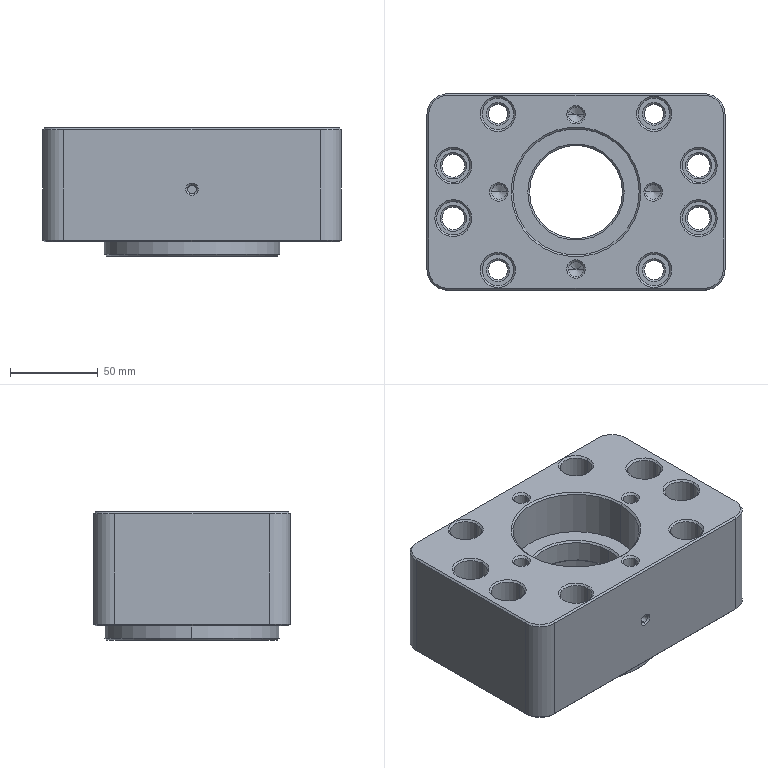NC program | NX | posted with a generic post | part box 170 x 112 x 73 mm
Lines 1 to 69 of 12198:
N10 G17 G21 G94 G90
(DRILLING , TOOL : ZXZ)
N12 T01 M6
N14 G54
N16 G17 G0 G90 X44.5 Y-44.5 S5000 M3
N18 G43 Z30. H1
N20 G94 G81 G98 Z-1. F250. R3.
N22 X70. Y-15.
N24 X44. Y0.
N26 X70. Y15.
N28 X44.5 Y44.5
N30 X0. Y44.
N32 Y0.
N34 Y-44.
N36 X-44.5 Y-44.5
N38 X-70. Y-15.
N40 X-44. Y0.
N42 X-70. Y15.
N44 X-44.5 Y44.5
N46 G80
N48 G0 X-44.5 Y44.5 Z30.
N50 M5
(DRILLING_COPY_COPY_1 , TOOL : 8.5ZT)
N52 T18 M6
N54 G54
N56 G17 G0 G90 X44. Y0. S1573 M3
N58 G43 Z30. H18
N60 G94 G83 G98 Z-28.054 F250. Q2. R3.
N62 X0. Y-44.
N64 X-44. Y0.
N66 X0. Y44.
N68 G80
N70 G0 X0. Y44. Z30.
N72 M5
(DRILLING_COPY_COPY_1_COPY , TOOL : 13.0ZT)
N74 T14 M6
N76 G54
N78 G17 G0 G90 X-70. Y-15. S700 M3
N80 G43 Z30. H14
N82 G94 G83 G98 Z-70.406 F150. Q3. R3.
N84 Y15.
N86 X0. Y0. Z-46.406
N88 X70. Y-15. Z-70.406
N90 Y15.
N92 G80
N94 G0 X70. Y15. Z30.
N96 M5
(DRILLING_COPY_COPY , TOOL : 11.0ZT)
N98 T11 M6
N100 G54
N102 G17 G0 G90 X44.5 Y-44.5 S1200 M3
N104 G43 Z30. H11
N106 G94 G83 G98 Z-69.805 F150. Q2. R3.
N108 X-44.5
N110 Y44.5
N112 X44.5
N114 G80
N116 G0 X44.5 Y44.5 Z30.
N118 M5